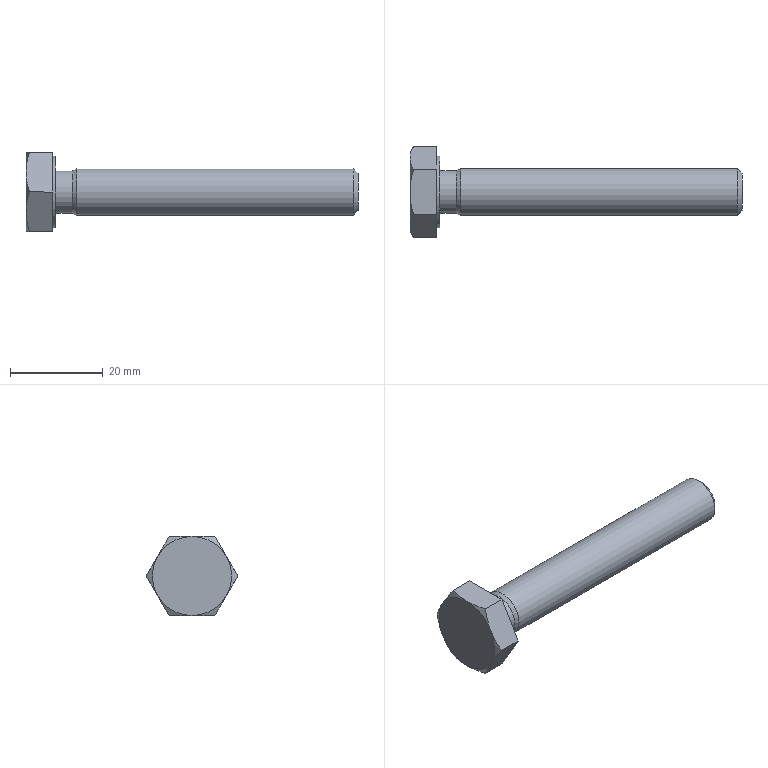Part | STEP file | DIN 933 - M10  x 65 | 1 solid | 21 faces | box 71.4 x 19.63 x 17 mm | volume 6601 mm3 | plane 10 | cone 8 | cylinder 3 | commonest cylinder face diameters 9.188 x1 10 x1 15.4 x1